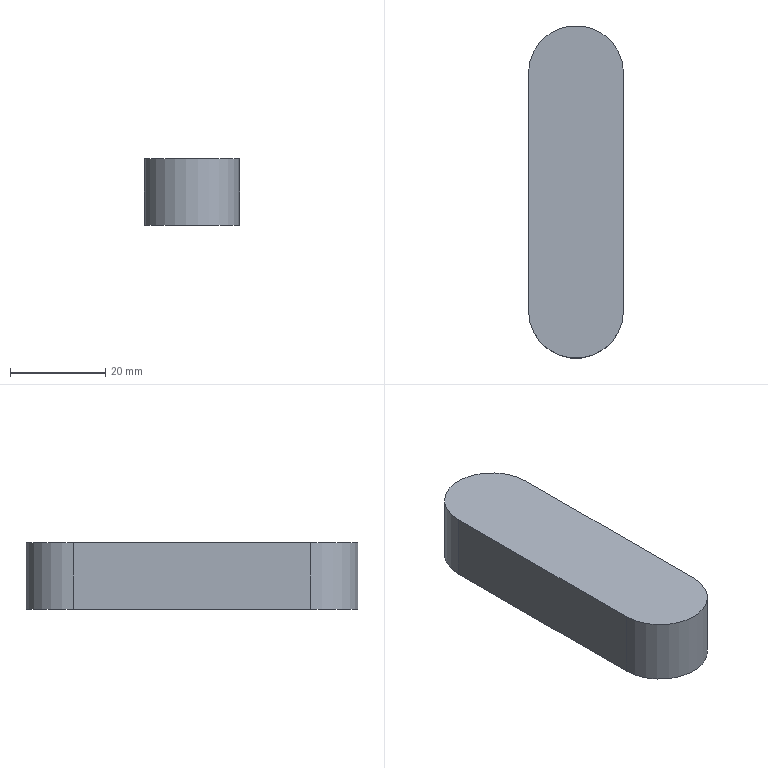Part | NX | 1 solid | 6 faces | box 20 x 70 x 14 mm | volume 18398 mm3 | plane 4 | cylinder 2 | commonest cylinder face diameters 20 x2
STEP:
#1=CARTESIAN_POINT('',(-10.,25.,14.));
#2=VERTEX_POINT('',#1);
#3=CARTESIAN_POINT('',(-10.,-25.,14.));
#4=VERTEX_POINT('',#3);
#5=CARTESIAN_POINT('',(-10.,35.,14.));
#6=DIRECTION('',(0.,-1.,0.));
#7=VECTOR('',#6,1.);
#8=LINE('',#5,#7);
#9=EDGE_CURVE('',#2,#4,#8,.T.);
#10=ORIENTED_EDGE('',*,*,#9,.F.);
#11=CARTESIAN_POINT('',(-10.,25.,0.));
#12=VERTEX_POINT('',#11);
#13=CARTESIAN_POINT('',(-10.,25.,14.));
#14=DIRECTION('',(0.,0.,-1.));
#15=VECTOR('',#14,1.);
#16=LINE('',#13,#15);
#17=EDGE_CURVE('',#2,#12,#16,.T.);
#18=ORIENTED_EDGE('',*,*,#17,.T.);
#19=CARTESIAN_POINT('',(-10.,-25.,0.));
#20=VERTEX_POINT('',#19);
#21=CARTESIAN_POINT('',(-10.,35.,0.));
#22=DIRECTION('',(0.,-1.,0.));
#23=VECTOR('',#22,1.);
#24=LINE('',#21,#23);
#25=EDGE_CURVE('',#12,#20,#24,.T.);
#26=ORIENTED_EDGE('',*,*,#25,.T.);
#27=CARTESIAN_POINT('',(-10.,-25.,14.));
#28=DIRECTION('',(0.,0.,1.));
#29=VECTOR('',#28,1.);
#30=LINE('',#27,#29);
#31=EDGE_CURVE('',#20,#4,#30,.T.);
#32=ORIENTED_EDGE('',*,*,#31,.T.);
#33=EDGE_LOOP('',(#10,#18,#26,#32));
#34=FACE_OUTER_BOUND('',#33,.T.);
#35=CARTESIAN_POINT('',(-10.,35.,14.));
#36=DIRECTION('',(1.,0.,0.));
#37=DIRECTION('',(0.,-1.,0.));
#38=AXIS2_PLACEMENT_3D('',#35,#36,#37);
#39=PLANE('',#38);
#40=ADVANCED_FACE('',(#34),#39,.F.);
#41=CARTESIAN_POINT('',(10.,-25.,0.));
#42=VERTEX_POINT('',#41);
#43=CARTESIAN_POINT('',(10.,25.,0.));
#44=VERTEX_POINT('',#43);
#45=CARTESIAN_POINT('',(10.,-35.,0.));
#46=DIRECTION('',(0.,1.,0.));
#47=VECTOR('',#46,1.);
#48=LINE('',#45,#47);
#49=EDGE_CURVE('',#42,#44,#48,.T.);
#50=ORIENTED_EDGE('',*,*,#49,.T.);
#51=CARTESIAN_POINT('',(10.,25.,14.));
#52=VERTEX_POINT('',#51);
#53=CARTESIAN_POINT('',(10.,25.,14.));
#54=DIRECTION('',(0.,0.,1.));
#55=VECTOR('',#54,1.);
#56=LINE('',#53,#55);
#57=EDGE_CURVE('',#44,#52,#56,.T.);
#58=ORIENTED_EDGE('',*,*,#57,.T.);
#59=CARTESIAN_POINT('',(10.,-25.,14.));
#60=VERTEX_POINT('',#59);
#61=CARTESIAN_POINT('',(10.,-35.,14.));
#62=DIRECTION('',(0.,1.,0.));
#63=VECTOR('',#62,1.);
#64=LINE('',#61,#63);
#65=EDGE_CURVE('',#60,#52,#64,.T.);
#66=ORIENTED_EDGE('',*,*,#65,.F.);
#67=CARTESIAN_POINT('',(10.,-25.,14.));
#68=DIRECTION('',(0.,0.,-1.));
#69=VECTOR('',#68,1.);
#70=LINE('',#67,#69);
#71=EDGE_CURVE('',#60,#42,#70,.T.);
#72=ORIENTED_EDGE('',*,*,#71,.T.);
#73=EDGE_LOOP('',(#50,#58,#66,#72));
#74=FACE_OUTER_BOUND('',#73,.T.);
#75=CARTESIAN_POINT('',(10.,-35.,14.));
#76=DIRECTION('',(-1.,0.,0.));
#77=DIRECTION('',(0.,1.,0.));
#78=AXIS2_PLACEMENT_3D('',#75,#76,#77);
#79=PLANE('',#78);
#80=ADVANCED_FACE('',(#74),#79,.F.);
#81=ORIENTED_EDGE('',*,*,#65,.T.);
#82=CARTESIAN_POINT('',(0.,25.,14.));
#83=DIRECTION('',(0.,0.,1.));
#84=DIRECTION('',(1.,0.,0.));
#85=AXIS2_PLACEMENT_3D('',#82,#83,#84);
#86=CIRCLE('',#85,10.);
#87=EDGE_CURVE('',#52,#2,#86,.T.);
#88=ORIENTED_EDGE('',*,*,#87,.T.);
#89=ORIENTED_EDGE('',*,*,#9,.T.);
#90=CARTESIAN_POINT('',(0.,-25.,14.));
#91=DIRECTION('',(0.,0.,1.));
#92=DIRECTION('',(1.,0.,0.));
#93=AXIS2_PLACEMENT_3D('',#90,#91,#92);
#94=CIRCLE('',#93,10.);
#95=EDGE_CURVE('',#4,#60,#94,.T.);
#96=ORIENTED_EDGE('',*,*,#95,.T.);
#97=EDGE_LOOP('',(#81,#88,#89,#96));
#98=FACE_OUTER_BOUND('',#97,.T.);
#99=CARTESIAN_POINT('',(0.,0.,14.));
#100=DIRECTION('',(0.,0.,1.));
#101=DIRECTION('',(-1.,0.,0.));
#102=AXIS2_PLACEMENT_3D('',#99,#100,#101);
#103=PLANE('',#102);
#104=ADVANCED_FACE('',(#98),#103,.T.);
#105=CARTESIAN_POINT('',(0.,25.,0.));
#106=DIRECTION('',(0.,0.,-1.));
#107=DIRECTION('',(1.,0.,0.));
#108=AXIS2_PLACEMENT_3D('',#105,#106,#107);
#109=CIRCLE('',#108,10.);
#110=EDGE_CURVE('',#12,#44,#109,.T.);
#111=ORIENTED_EDGE('',*,*,#110,.T.);
#112=ORIENTED_EDGE('',*,*,#49,.F.);
#113=CARTESIAN_POINT('',(0.,-25.,0.));
#114=DIRECTION('',(0.,0.,-1.));
#115=DIRECTION('',(1.,0.,0.));
#116=AXIS2_PLACEMENT_3D('',#113,#114,#115);
#117=CIRCLE('',#116,10.);
#118=EDGE_CURVE('',#42,#20,#117,.T.);
#119=ORIENTED_EDGE('',*,*,#118,.T.);
#120=ORIENTED_EDGE('',*,*,#25,.F.);
#121=EDGE_LOOP('',(#111,#112,#119,#120));
#122=FACE_OUTER_BOUND('',#121,.T.);
#123=CARTESIAN_POINT('',(0.,0.,0.));
#124=DIRECTION('',(0.,0.,1.));
#125=DIRECTION('',(-1.,0.,0.));
#126=AXIS2_PLACEMENT_3D('',#123,#124,#125);
#127=PLANE('',#126);
#128=ADVANCED_FACE('',(#122),#127,.F.);
#129=ORIENTED_EDGE('',*,*,#17,.F.);
#130=ORIENTED_EDGE('',*,*,#87,.F.);
#131=ORIENTED_EDGE('',*,*,#57,.F.);
#132=ORIENTED_EDGE('',*,*,#110,.F.);
#133=EDGE_LOOP('',(#129,#130,#131,#132));
#134=FACE_OUTER_BOUND('',#133,.T.);
#135=CARTESIAN_POINT('',(0.,25.,14.));
#136=DIRECTION('',(0.,0.,-1.));
#137=DIRECTION('',(1.,0.,0.));
#138=AXIS2_PLACEMENT_3D('',#135,#136,#137);
#139=CYLINDRICAL_SURFACE('',#138,10.);
#140=ADVANCED_FACE('',(#134),#139,.T.);
#141=ORIENTED_EDGE('',*,*,#118,.F.);
#142=ORIENTED_EDGE('',*,*,#71,.F.);
#143=ORIENTED_EDGE('',*,*,#95,.F.);
#144=ORIENTED_EDGE('',*,*,#31,.F.);
#145=EDGE_LOOP('',(#141,#142,#143,#144));
#146=FACE_OUTER_BOUND('',#145,.T.);
#147=CARTESIAN_POINT('',(0.,-25.,14.));
#148=DIRECTION('',(0.,0.,-1.));
#149=DIRECTION('',(1.,0.,0.));
#150=AXIS2_PLACEMENT_3D('',#147,#148,#149);
#151=CYLINDRICAL_SURFACE('',#150,10.);
#152=ADVANCED_FACE('',(#146),#151,.T.);
#153=CLOSED_SHELL('',(#40,#80,#104,#128,#140,#152));
#154=MANIFOLD_SOLID_BREP('',#153);
#155=(LENGTH_UNIT()NAMED_UNIT(*)SI_UNIT(.MILLI.,.METRE.));
#156=UNCERTAINTY_MEASURE_WITH_UNIT(LENGTH_MEASURE(0.00002),#155,'','');
#157=(NAMED_UNIT(*)PLANE_ANGLE_UNIT()SI_UNIT($,.RADIAN.));
#158=PLANE_ANGLE_MEASURE_WITH_UNIT(PLANE_ANGLE_MEASURE(0.01745),#157);
#159=DIMENSIONAL_EXPONENTS(0.,0.,0.,0.,0.,0.,0.);
#160=(CONVERSION_BASED_UNIT('DEGREE',#158)NAMED_UNIT(#159)PLANE_ANGLE_UNIT());
#161=(NAMED_UNIT(*)SI_UNIT($,.STERADIAN.)SOLID_ANGLE_UNIT());
#162=(GEOMETRIC_REPRESENTATION_CONTEXT(3)GLOBAL_UNCERTAINTY_ASSIGNED_CONTEXT((#156))GLOBAL_UNIT_ASSIGNED_CONTEXT((#155,#160,#161))REPRESENTATION_CONTEXT('',''));
#163=ADVANCED_BREP_SHAPE_REPRESENTATION('',(#154),#162);